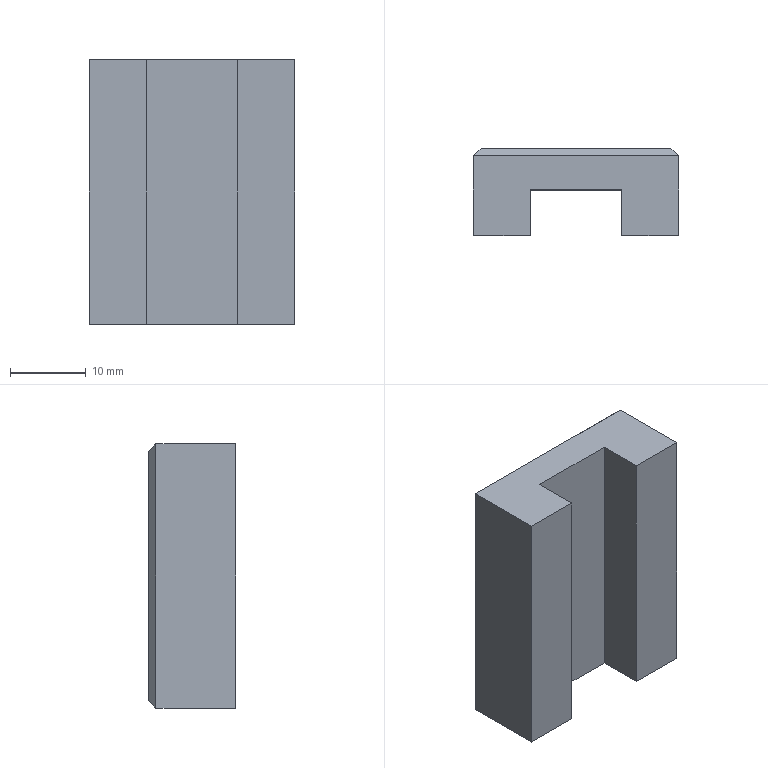Part | STEP file | BMC12B slider | 1 solid | 30 faces | box 27 x 11.5 x 34.8 mm | volume 8068 mm3 | plane 14 | cylinder 8 | cone 8 | commonest cylinder face diameters 2.5 x8